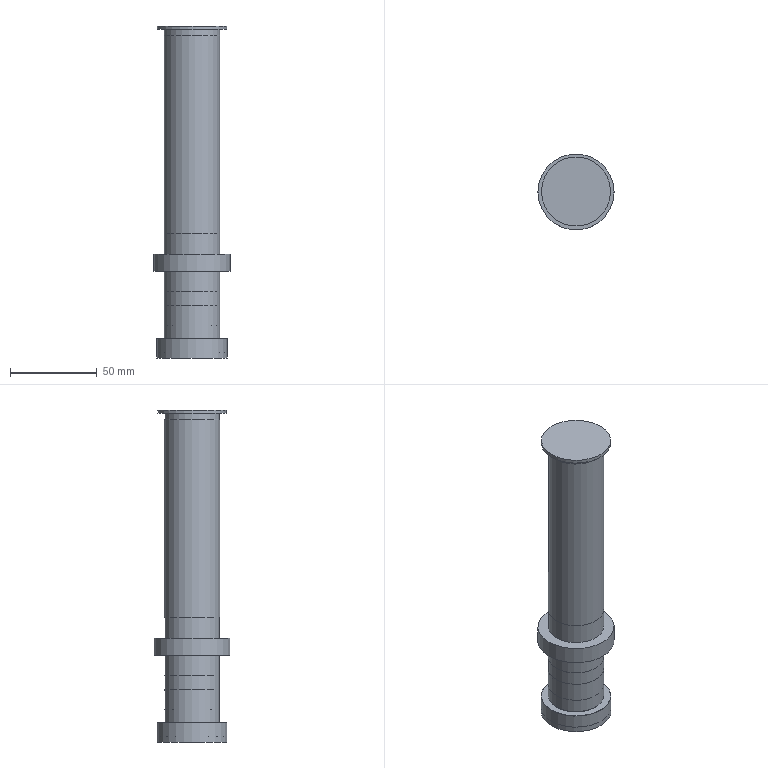Part | NX | features BREP 4 | 4 solids | 41 faces | box 44 x 44 x 191.85 mm | volume 315656 mm3 | plane 19 | cylinder 18 | torus 2 | cone 2 | commonest cylinder face diameters 8 x2 10 x2 14 x2 32 x2 40 x2 44 x2
STEP:
#1=CARTESIAN_POINT('',(-4.,0.,139.85));
#2=VERTEX_POINT('',#1);
#3=CARTESIAN_POINT('',(0.,0.,139.85));
#4=DIRECTION('',(0.,0.,1.));
#5=DIRECTION('',(-1.,0.,0.));
#6=AXIS2_PLACEMENT_3D('',#3,#4,#5);
#7=CIRCLE('',#6,4.);
#8=EDGE_CURVE('',#2,#2,#7,.T.);
#9=ORIENTED_EDGE('',*,*,#8,.F.);
#10=EDGE_LOOP('',(#9));
#11=FACE_BOUND('',#10,.T.);
#12=CARTESIAN_POINT('',(-4.,0.,134.85));
#13=VERTEX_POINT('',#12);
#14=CARTESIAN_POINT('',(0.,0.,134.85));
#15=DIRECTION('',(0.,0.,1.));
#16=DIRECTION('',(-1.,0.,0.));
#17=AXIS2_PLACEMENT_3D('',#14,#15,#16);
#18=CIRCLE('',#17,4.);
#19=EDGE_CURVE('',#13,#13,#18,.T.);
#20=ORIENTED_EDGE('',*,*,#19,.T.);
#21=EDGE_LOOP('',(#20));
#22=FACE_BOUND('',#21,.T.);
#23=CARTESIAN_POINT('',(0.,0.,139.85));
#24=DIRECTION('',(0.,0.,-1.));
#25=DIRECTION('',(1.,0.,0.));
#26=AXIS2_PLACEMENT_3D('',#23,#24,#25);
#27=CYLINDRICAL_SURFACE('',#26,4.);
#28=ADVANCED_FACE('',(#11,#22),#27,.T.);
#29=ORIENTED_EDGE('',*,*,#19,.F.);
#30=EDGE_LOOP('',(#29));
#31=FACE_BOUND('',#30,.T.);
#32=CARTESIAN_POINT('',(0.,0.,134.85));
#33=DIRECTION('',(0.,0.,1.));
#34=DIRECTION('',(-1.,0.,0.));
#35=AXIS2_PLACEMENT_3D('',#32,#33,#34);
#36=PLANE('',#35);
#37=ADVANCED_FACE('',(#31),#36,.F.);
#38=CARTESIAN_POINT('',(20.,0.,139.85));
#39=VERTEX_POINT('',#38);
#40=CARTESIAN_POINT('',(0.,0.,139.85));
#41=DIRECTION('',(0.,0.,1.));
#42=DIRECTION('',(1.,0.,0.));
#43=AXIS2_PLACEMENT_3D('',#40,#41,#42);
#44=CIRCLE('',#43,20.);
#45=EDGE_CURVE('',#39,#39,#44,.T.);
#46=ORIENTED_EDGE('',*,*,#45,.F.);
#47=EDGE_LOOP('',(#46));
#48=FACE_BOUND('',#47,.T.);
#49=ORIENTED_EDGE('',*,*,#8,.T.);
#50=EDGE_LOOP('',(#49));
#51=FACE_BOUND('',#50,.T.);
#52=CARTESIAN_POINT('',(0.,0.,139.85));
#53=DIRECTION('',(0.,0.,-1.));
#54=DIRECTION('',(1.,0.,0.));
#55=AXIS2_PLACEMENT_3D('',#52,#53,#54);
#56=PLANE('',#55);
#57=ADVANCED_FACE('',(#48,#51),#56,.T.);
#58=CARTESIAN_POINT('',(20.,0.,141.85));
#59=VERTEX_POINT('',#58);
#60=CARTESIAN_POINT('',(0.,0.,141.85));
#61=DIRECTION('',(0.,0.,1.));
#62=DIRECTION('',(1.,0.,0.));
#63=AXIS2_PLACEMENT_3D('',#60,#61,#62);
#64=CIRCLE('',#63,20.);
#65=EDGE_CURVE('',#59,#59,#64,.T.);
#66=ORIENTED_EDGE('',*,*,#65,.T.);
#67=EDGE_LOOP('',(#66));
#68=FACE_BOUND('',#67,.T.);
#69=CARTESIAN_POINT('',(0.,0.,141.85));
#70=DIRECTION('',(0.,0.,1.));
#71=DIRECTION('',(-1.,0.,0.));
#72=AXIS2_PLACEMENT_3D('',#69,#70,#71);
#73=PLANE('',#72);
#74=ADVANCED_FACE('',(#68),#73,.T.);
#75=ORIENTED_EDGE('',*,*,#65,.F.);
#76=EDGE_LOOP('',(#75));
#77=FACE_BOUND('',#76,.T.);
#78=ORIENTED_EDGE('',*,*,#45,.T.);
#79=EDGE_LOOP('',(#78));
#80=FACE_BOUND('',#79,.T.);
#81=CARTESIAN_POINT('',(0.,0.,139.85));
#82=DIRECTION('',(0.,0.,1.));
#83=DIRECTION('',(-1.,0.,0.));
#84=AXIS2_PLACEMENT_3D('',#81,#82,#83);
#85=CYLINDRICAL_SURFACE('',#84,20.);
#86=ADVANCED_FACE('',(#77,#80),#85,.T.);
#87=CLOSED_SHELL('',(#28,#37,#57,#74,#86));
#88=MANIFOLD_SOLID_BREP('',#87);
#89=CARTESIAN_POINT('',(16.,0.,0.));
#90=VERTEX_POINT('',#89);
#91=CARTESIAN_POINT('',(0.,0.,0.));
#92=DIRECTION('',(0.,0.,1.));
#93=DIRECTION('',(1.,0.,0.));
#94=AXIS2_PLACEMENT_3D('',#91,#92,#93);
#95=CIRCLE('',#94,16.);
#96=EDGE_CURVE('',#90,#90,#95,.T.);
#97=ORIENTED_EDGE('',*,*,#96,.F.);
#98=EDGE_LOOP('',(#97));
#99=FACE_BOUND('',#98,.T.);
#100=CARTESIAN_POINT('',(-16.,0.,-39.));
#101=VERTEX_POINT('',#100);
#102=CARTESIAN_POINT('',(0.,0.,-39.));
#103=DIRECTION('',(0.,0.,-1.));
#104=DIRECTION('',(-1.,0.,0.));
#105=AXIS2_PLACEMENT_3D('',#102,#103,#104);
#106=CIRCLE('',#105,16.);
#107=EDGE_CURVE('',#101,#101,#106,.T.);
#108=ORIENTED_EDGE('',*,*,#107,.F.);
#109=EDGE_LOOP('',(#108));
#110=FACE_BOUND('',#109,.T.);
#111=CARTESIAN_POINT('',(0.,0.,-23.));
#112=DIRECTION('',(0.,0.,1.));
#113=DIRECTION('',(-1.,0.,0.));
#114=AXIS2_PLACEMENT_3D('',#111,#112,#113);
#115=CYLINDRICAL_SURFACE('',#114,16.);
#116=ADVANCED_FACE('',(#99,#110),#115,.T.);
#117=CARTESIAN_POINT('',(-20.25,0.,-50.));
#118=VERTEX_POINT('',#117);
#119=CARTESIAN_POINT('',(0.,0.,-50.));
#120=DIRECTION('',(0.,0.,-1.));
#121=DIRECTION('',(-1.,0.,0.));
#122=AXIS2_PLACEMENT_3D('',#119,#120,#121);
#123=CIRCLE('',#122,20.25);
#124=EDGE_CURVE('',#118,#118,#123,.T.);
#125=ORIENTED_EDGE('',*,*,#124,.T.);
#126=EDGE_LOOP('',(#125));
#127=FACE_BOUND('',#126,.T.);
#128=CARTESIAN_POINT('',(0.,0.,-50.));
#129=DIRECTION('',(0.,0.,-1.));
#130=DIRECTION('',(1.,0.,0.));
#131=AXIS2_PLACEMENT_3D('',#128,#129,#130);
#132=PLANE('',#131);
#133=ADVANCED_FACE('',(#127),#132,.T.);
#134=ORIENTED_EDGE('',*,*,#107,.T.);
#135=EDGE_LOOP('',(#134));
#136=FACE_BOUND('',#135,.T.);
#137=CARTESIAN_POINT('',(-20.25,0.,-39.));
#138=VERTEX_POINT('',#137);
#139=CARTESIAN_POINT('',(0.,0.,-39.));
#140=DIRECTION('',(0.,0.,-1.));
#141=DIRECTION('',(-1.,0.,0.));
#142=AXIS2_PLACEMENT_3D('',#139,#140,#141);
#143=CIRCLE('',#142,20.25);
#144=EDGE_CURVE('',#138,#138,#143,.T.);
#145=ORIENTED_EDGE('',*,*,#144,.F.);
#146=EDGE_LOOP('',(#145));
#147=FACE_BOUND('',#146,.T.);
#148=CARTESIAN_POINT('',(0.,0.,-39.));
#149=DIRECTION('',(0.,0.,1.));
#150=DIRECTION('',(-1.,0.,0.));
#151=AXIS2_PLACEMENT_3D('',#148,#149,#150);
#152=PLANE('',#151);
#153=ADVANCED_FACE('',(#136,#147),#152,.T.);
#154=ORIENTED_EDGE('',*,*,#124,.F.);
#155=EDGE_LOOP('',(#154));
#156=FACE_BOUND('',#155,.T.);
#157=ORIENTED_EDGE('',*,*,#144,.T.);
#158=EDGE_LOOP('',(#157));
#159=FACE_BOUND('',#158,.T.);
#160=CARTESIAN_POINT('',(0.,0.,-39.));
#161=DIRECTION('',(0.,0.,-1.));
#162=DIRECTION('',(1.,0.,0.));
#163=AXIS2_PLACEMENT_3D('',#160,#161,#162);
#164=CYLINDRICAL_SURFACE('',#163,20.25);
#165=ADVANCED_FACE('',(#156,#159),#164,.T.);
#166=CARTESIAN_POINT('',(16.,0.,10.));
#167=VERTEX_POINT('',#166);
#168=CARTESIAN_POINT('',(0.,0.,10.));
#169=DIRECTION('',(0.,0.,1.));
#170=DIRECTION('',(1.,0.,0.));
#171=AXIS2_PLACEMENT_3D('',#168,#169,#170);
#172=CIRCLE('',#171,16.);
#173=EDGE_CURVE('',#167,#167,#172,.T.);
#174=ORIENTED_EDGE('',*,*,#173,.F.);
#175=EDGE_LOOP('',(#174));
#176=FACE_BOUND('',#175,.T.);
#177=CARTESIAN_POINT('',(22.,0.,10.));
#178=VERTEX_POINT('',#177);
#179=CARTESIAN_POINT('',(0.,0.,10.));
#180=DIRECTION('',(0.,0.,1.));
#181=DIRECTION('',(1.,0.,0.));
#182=AXIS2_PLACEMENT_3D('',#179,#180,#181);
#183=CIRCLE('',#182,22.);
#184=EDGE_CURVE('',#178,#178,#183,.T.);
#185=ORIENTED_EDGE('',*,*,#184,.T.);
#186=EDGE_LOOP('',(#185));
#187=FACE_BOUND('',#186,.T.);
#188=CARTESIAN_POINT('',(0.,0.,10.));
#189=DIRECTION('',(0.,0.,1.));
#190=DIRECTION('',(-1.,0.,0.));
#191=AXIS2_PLACEMENT_3D('',#188,#189,#190);
#192=PLANE('',#191);
#193=ADVANCED_FACE('',(#176,#187),#192,.T.);
#194=ORIENTED_EDGE('',*,*,#96,.T.);
#195=EDGE_LOOP('',(#194));
#196=FACE_BOUND('',#195,.T.);
#197=CARTESIAN_POINT('',(22.,0.,0.));
#198=VERTEX_POINT('',#197);
#199=CARTESIAN_POINT('',(0.,0.,0.));
#200=DIRECTION('',(0.,0.,1.));
#201=DIRECTION('',(1.,0.,0.));
#202=AXIS2_PLACEMENT_3D('',#199,#200,#201);
#203=CIRCLE('',#202,22.);
#204=EDGE_CURVE('',#198,#198,#203,.T.);
#205=ORIENTED_EDGE('',*,*,#204,.F.);
#206=EDGE_LOOP('',(#205));
#207=FACE_BOUND('',#206,.T.);
#208=CARTESIAN_POINT('',(0.,0.,0.));
#209=DIRECTION('',(0.,0.,-1.));
#210=DIRECTION('',(1.,0.,0.));
#211=AXIS2_PLACEMENT_3D('',#208,#209,#210);
#212=PLANE('',#211);
#213=ADVANCED_FACE('',(#196,#207),#212,.T.);
#214=ORIENTED_EDGE('',*,*,#184,.F.);
#215=EDGE_LOOP('',(#214));
#216=FACE_BOUND('',#215,.T.);
#217=ORIENTED_EDGE('',*,*,#204,.T.);
#218=EDGE_LOOP('',(#217));
#219=FACE_BOUND('',#218,.T.);
#220=CARTESIAN_POINT('',(0.,0.,0.));
#221=DIRECTION('',(0.,0.,1.));
#222=DIRECTION('',(-1.,0.,0.));
#223=AXIS2_PLACEMENT_3D('',#220,#221,#222);
#224=CYLINDRICAL_SURFACE('',#223,22.);
#225=ADVANCED_FACE('',(#216,#219),#224,.T.);
#226=CARTESIAN_POINT('',(16.,0.,139.85));
#227=VERTEX_POINT('',#226);
#228=CARTESIAN_POINT('',(0.,0.,139.85));
#229=DIRECTION('',(0.,0.,1.));
#230=DIRECTION('',(1.,0.,0.));
#231=AXIS2_PLACEMENT_3D('',#228,#229,#230);
#232=CIRCLE('',#231,16.);
#233=EDGE_CURVE('',#227,#227,#232,.T.);
#234=ORIENTED_EDGE('',*,*,#233,.T.);
#235=EDGE_LOOP('',(#234));
#236=FACE_BOUND('',#235,.T.);
#237=CARTESIAN_POINT('',(0.,0.,139.85));
#238=DIRECTION('',(0.,0.,1.));
#239=DIRECTION('',(-1.,0.,0.));
#240=AXIS2_PLACEMENT_3D('',#237,#238,#239);
#241=PLANE('',#240);
#242=ADVANCED_FACE('',(#236),#241,.T.);
#243=ORIENTED_EDGE('',*,*,#233,.F.);
#244=EDGE_LOOP('',(#243));
#245=FACE_BOUND('',#244,.T.);
#246=ORIENTED_EDGE('',*,*,#173,.T.);
#247=EDGE_LOOP('',(#246));
#248=FACE_BOUND('',#247,.T.);
#249=CARTESIAN_POINT('',(0.,0.,10.));
#250=DIRECTION('',(0.,0.,1.));
#251=DIRECTION('',(-1.,0.,0.));
#252=AXIS2_PLACEMENT_3D('',#249,#250,#251);
#253=CYLINDRICAL_SURFACE('',#252,16.);
#254=ADVANCED_FACE('',(#245,#248),#253,.T.);
#255=CLOSED_SHELL('',(#116,#133,#153,#165,#193,#213,#225,#242,#254));
#256=MANIFOLD_SOLID_BREP('',#255);
#257=CARTESIAN_POINT('',(-7.,0.,139.85));
#258=VERTEX_POINT('',#257);
#259=CARTESIAN_POINT('',(0.,0.,139.85));
#260=DIRECTION('',(0.,0.,-1.));
#261=DIRECTION('',(-1.,0.,0.));
#262=AXIS2_PLACEMENT_3D('',#259,#260,#261);
#263=CIRCLE('',#262,7.);
#264=EDGE_CURVE('',#258,#258,#263,.T.);
#265=ORIENTED_EDGE('',*,*,#264,.T.);
#266=EDGE_LOOP('',(#265));
#267=FACE_BOUND('',#266,.T.);
#268=CARTESIAN_POINT('',(12.509,0.,139.85));
#269=VERTEX_POINT('',#268);
#270=CARTESIAN_POINT('',(0.,0.,139.85));
#271=DIRECTION('',(0.,0.,1.));
#272=DIRECTION('',(1.,0.,0.));
#273=AXIS2_PLACEMENT_3D('',#270,#271,#272);
#274=CIRCLE('',#273,12.509);
#275=EDGE_CURVE('',#269,#269,#274,.T.);
#276=ORIENTED_EDGE('',*,*,#275,.T.);
#277=EDGE_LOOP('',(#276));
#278=FACE_BOUND('',#277,.T.);
#279=CARTESIAN_POINT('',(0.,0.,139.85));
#280=DIRECTION('',(0.,0.,1.));
#281=DIRECTION('',(-1.,0.,0.));
#282=AXIS2_PLACEMENT_3D('',#279,#280,#281);
#283=PLANE('',#282);
#284=ADVANCED_FACE('',(#267,#278),#283,.T.);
#285=CARTESIAN_POINT('',(16.009,0.,22.));
#286=VERTEX_POINT('',#285);
#287=CARTESIAN_POINT('',(0.,0.,22.));
#288=DIRECTION('',(0.,0.,-1.));
#289=DIRECTION('',(1.,0.,0.));
#290=AXIS2_PLACEMENT_3D('',#287,#288,#289);
#291=CIRCLE('',#290,16.009);
#292=EDGE_CURVE('',#286,#286,#291,.T.);
#293=ORIENTED_EDGE('',*,*,#292,.F.);
#294=EDGE_LOOP('',(#293));
#295=FACE_BOUND('',#294,.T.);
#296=CARTESIAN_POINT('',(16.009,0.,136.35));
#297=VERTEX_POINT('',#296);
#298=CARTESIAN_POINT('',(0.,0.,136.35));
#299=DIRECTION('',(0.,0.,-1.));
#300=DIRECTION('',(1.,0.,0.));
#301=AXIS2_PLACEMENT_3D('',#298,#299,#300);
#302=CIRCLE('',#301,16.009);
#303=EDGE_CURVE('',#297,#297,#302,.T.);
#304=ORIENTED_EDGE('',*,*,#303,.T.);
#305=EDGE_LOOP('',(#304));
#306=FACE_BOUND('',#305,.T.);
#307=CARTESIAN_POINT('',(0.,0.,10.));
#308=DIRECTION('',(0.,0.,1.));
#309=DIRECTION('',(-1.,0.,0.));
#310=AXIS2_PLACEMENT_3D('',#307,#308,#309);
#311=CYLINDRICAL_SURFACE('',#310,16.009);
#312=ADVANCED_FACE('',(#295,#306),#311,.T.);
#313=ORIENTED_EDGE('',*,*,#303,.F.);
#314=EDGE_LOOP('',(#313));
#315=FACE_BOUND('',#314,.T.);
#316=ORIENTED_EDGE('',*,*,#275,.F.);
#317=EDGE_LOOP('',(#316));
#318=FACE_BOUND('',#317,.T.);
#319=CARTESIAN_POINT('',(0.,0.,136.35));
#320=DIRECTION('',(0.,0.,1.));
#321=DIRECTION('',(-1.,0.,0.));
#322=AXIS2_PLACEMENT_3D('',#319,#320,#321);
#323=TOROIDAL_SURFACE('',#322,12.509,3.5);
#324=ADVANCED_FACE('',(#315,#318),#323,.T.);
#325=CARTESIAN_POINT('',(-4.,0.,114.85));
#326=VERTEX_POINT('',#325);
#327=CARTESIAN_POINT('',(0.,0.,114.85));
#328=DIRECTION('',(0.,0.,-1.));
#329=DIRECTION('',(-1.,0.,0.));
#330=AXIS2_PLACEMENT_3D('',#327,#328,#329);
#331=CIRCLE('',#330,4.);
#332=EDGE_CURVE('',#326,#326,#331,.T.);
#333=ORIENTED_EDGE('',*,*,#332,.F.);
#334=EDGE_LOOP('',(#333));
#335=FACE_BOUND('',#334,.T.);
#336=CARTESIAN_POINT('',(0.,0.,112.447));
#337=VERTEX_POINT('',#336);
#338=VERTEX_LOOP('',#337);
#339=FACE_BOUND('',#338,.T.);
#340=CARTESIAN_POINT('',(0.,0.,114.85));
#341=DIRECTION('',(0.,0.,1.));
#342=DIRECTION('',(-1.,0.,0.));
#343=AXIS2_PLACEMENT_3D('',#340,#341,#342);
#344=CONICAL_SURFACE('',#343,4.,1.03);
#345=ADVANCED_FACE('',(#335,#339),#344,.F.);
#346=ORIENTED_EDGE('',*,*,#332,.T.);
#347=EDGE_LOOP('',(#346));
#348=FACE_BOUND('',#347,.T.);
#349=CARTESIAN_POINT('',(-4.,0.,134.85));
#350=VERTEX_POINT('',#349);
#351=CARTESIAN_POINT('',(0.,0.,134.85));
#352=DIRECTION('',(0.,0.,-1.));
#353=DIRECTION('',(-1.,0.,0.));
#354=AXIS2_PLACEMENT_3D('',#351,#352,#353);
#355=CIRCLE('',#354,4.);
#356=EDGE_CURVE('',#350,#350,#355,.T.);
#357=ORIENTED_EDGE('',*,*,#356,.F.);
#358=EDGE_LOOP('',(#357));
#359=FACE_BOUND('',#358,.T.);
#360=CARTESIAN_POINT('',(0.,0.,114.85));
#361=DIRECTION('',(0.,0.,-1.));
#362=DIRECTION('',(1.,0.,0.));
#363=AXIS2_PLACEMENT_3D('',#360,#361,#362);
#364=CYLINDRICAL_SURFACE('',#363,4.);
#365=ADVANCED_FACE('',(#348,#359),#364,.F.);
#366=ORIENTED_EDGE('',*,*,#356,.T.);
#367=EDGE_LOOP('',(#366));
#368=FACE_BOUND('',#367,.T.);
#369=CARTESIAN_POINT('',(-7.,0.,134.85));
#370=VERTEX_POINT('',#369);
#371=CARTESIAN_POINT('',(0.,0.,134.85));
#372=DIRECTION('',(0.,0.,-1.));
#373=DIRECTION('',(-1.,0.,0.));
#374=AXIS2_PLACEMENT_3D('',#371,#372,#373);
#375=CIRCLE('',#374,7.);
#376=EDGE_CURVE('',#370,#370,#375,.T.);
#377=ORIENTED_EDGE('',*,*,#376,.F.);
#378=EDGE_LOOP('',(#377));
#379=FACE_BOUND('',#378,.T.);
#380=CARTESIAN_POINT('',(0.,0.,134.85));
#381=DIRECTION('',(0.,0.,-1.));
#382=DIRECTION('',(1.,0.,0.));
#383=AXIS2_PLACEMENT_3D('',#380,#381,#382);
#384=PLANE('',#383);
#385=ADVANCED_FACE('',(#368,#379),#384,.F.);
#386=ORIENTED_EDGE('',*,*,#376,.T.);
#387=EDGE_LOOP('',(#386));
#388=FACE_BOUND('',#387,.T.);
#389=ORIENTED_EDGE('',*,*,#264,.F.);
#390=EDGE_LOOP('',(#389));
#391=FACE_BOUND('',#390,.T.);
#392=CARTESIAN_POINT('',(0.,0.,139.85));
#393=DIRECTION('',(0.,0.,-1.));
#394=DIRECTION('',(1.,0.,0.));
#395=AXIS2_PLACEMENT_3D('',#392,#393,#394);
#396=CYLINDRICAL_SURFACE('',#395,7.);
#397=ADVANCED_FACE('',(#388,#391),#396,.F.);
#398=CARTESIAN_POINT('',(15.208,0.,22.));
#399=VERTEX_POINT('',#398);
#400=CARTESIAN_POINT('',(0.,0.,22.));
#401=DIRECTION('',(0.,0.,1.));
#402=DIRECTION('',(1.,0.,0.));
#403=AXIS2_PLACEMENT_3D('',#400,#401,#402);
#404=CIRCLE('',#403,15.208);
#405=EDGE_CURVE('',#399,#399,#404,.T.);
#406=ORIENTED_EDGE('',*,*,#405,.F.);
#407=EDGE_LOOP('',(#406));
#408=FACE_BOUND('',#407,.T.);
#409=CARTESIAN_POINT('',(15.208,0.,10.));
#410=VERTEX_POINT('',#409);
#411=CARTESIAN_POINT('',(0.,0.,10.));
#412=DIRECTION('',(0.,0.,1.));
#413=DIRECTION('',(1.,0.,0.));
#414=AXIS2_PLACEMENT_3D('',#411,#412,#413);
#415=CIRCLE('',#414,15.208);
#416=EDGE_CURVE('',#410,#410,#415,.T.);
#417=ORIENTED_EDGE('',*,*,#416,.T.);
#418=EDGE_LOOP('',(#417));
#419=FACE_BOUND('',#418,.T.);
#420=CARTESIAN_POINT('',(0.,0.,16.));
#421=DIRECTION('',(0.,0.,1.));
#422=DIRECTION('',(-1.,0.,0.));
#423=AXIS2_PLACEMENT_3D('',#420,#421,#422);
#424=CYLINDRICAL_SURFACE('',#423,15.208);
#425=ADVANCED_FACE('',(#408,#419),#424,.T.);
#426=ORIENTED_EDGE('',*,*,#292,.T.);
#427=EDGE_LOOP('',(#426));
#428=FACE_BOUND('',#427,.T.);
#429=ORIENTED_EDGE('',*,*,#405,.T.);
#430=EDGE_LOOP('',(#429));
#431=FACE_BOUND('',#430,.T.);
#432=CARTESIAN_POINT('',(0.,0.,22.));
#433=DIRECTION('',(0.,0.,1.));
#434=DIRECTION('',(-1.,0.,0.));
#435=AXIS2_PLACEMENT_3D('',#432,#433,#434);
#436=PLANE('',#435);
#437=ADVANCED_FACE('',(#428,#431),#436,.F.);
#438=CARTESIAN_POINT('',(-15.999,0.,0.));
#439=VERTEX_POINT('',#438);
#440=CARTESIAN_POINT('',(0.,0.,0.));
#441=DIRECTION('',(0.,0.,-1.));
#442=DIRECTION('',(-1.,0.,0.));
#443=AXIS2_PLACEMENT_3D('',#440,#441,#442);
#444=CIRCLE('',#443,15.999);
#445=EDGE_CURVE('',#439,#439,#444,.T.);
#446=ORIENTED_EDGE('',*,*,#445,.F.);
#447=EDGE_LOOP('',(#446));
#448=FACE_BOUND('',#447,.T.);
#449=CARTESIAN_POINT('',(22.,0.,0.));
#450=VERTEX_POINT('',#449);
#451=CARTESIAN_POINT('',(0.,0.,0.));
#452=DIRECTION('',(0.,0.,1.));
#453=DIRECTION('',(1.,0.,0.));
#454=AXIS2_PLACEMENT_3D('',#451,#452,#453);
#455=CIRCLE('',#454,22.);
#456=EDGE_CURVE('',#450,#450,#455,.T.);
#457=ORIENTED_EDGE('',*,*,#456,.F.);
#458=EDGE_LOOP('',(#457));
#459=FACE_BOUND('',#458,.T.);
#460=CARTESIAN_POINT('',(0.,0.,0.));
#461=DIRECTION('',(0.,0.,1.));
#462=DIRECTION('',(-1.,0.,0.));
#463=AXIS2_PLACEMENT_3D('',#460,#461,#462);
#464=PLANE('',#463);
#465=ADVANCED_FACE('',(#448,#459),#464,.F.);
#466=CARTESIAN_POINT('',(22.,0.,10.));
#467=VERTEX_POINT('',#466);
#468=CARTESIAN_POINT('',(0.,0.,10.));
#469=DIRECTION('',(0.,0.,1.));
#470=DIRECTION('',(1.,0.,0.));
#471=AXIS2_PLACEMENT_3D('',#468,#469,#470);
#472=CIRCLE('',#471,22.);
#473=EDGE_CURVE('',#467,#467,#472,.T.);
#474=ORIENTED_EDGE('',*,*,#473,.F.);
#475=EDGE_LOOP('',(#474));
#476=FACE_BOUND('',#475,.T.);
#477=ORIENTED_EDGE('',*,*,#456,.T.);
#478=EDGE_LOOP('',(#477));
#479=FACE_BOUND('',#478,.T.);
#480=CARTESIAN_POINT('',(0.,0.,10.));
#481=DIRECTION('',(0.,0.,-1.));
#482=DIRECTION('',(1.,0.,0.));
#483=AXIS2_PLACEMENT_3D('',#480,#481,#482);
#484=CYLINDRICAL_SURFACE('',#483,22.);
#485=ADVANCED_FACE('',(#476,#479),#484,.T.);
#486=ORIENTED_EDGE('',*,*,#473,.T.);
#487=EDGE_LOOP('',(#486));
#488=FACE_BOUND('',#487,.T.);
#489=ORIENTED_EDGE('',*,*,#416,.F.);
#490=EDGE_LOOP('',(#489));
#491=FACE_BOUND('',#490,.T.);
#492=CARTESIAN_POINT('',(0.,0.,10.));
#493=DIRECTION('',(0.,0.,1.));
#494=DIRECTION('',(-1.,0.,0.));
#495=AXIS2_PLACEMENT_3D('',#492,#493,#494);
#496=PLANE('',#495);
#497=ADVANCED_FACE('',(#488,#491),#496,.T.);
#498=CARTESIAN_POINT('',(-15.98,0.,-11.5));
#499=VERTEX_POINT('',#498);
#500=CARTESIAN_POINT('',(0.,0.,-11.5));
#501=DIRECTION('',(0.,0.,-1.));
#502=DIRECTION('',(-1.,0.,0.));
#503=AXIS2_PLACEMENT_3D('',#500,#501,#502);
#504=CIRCLE('',#503,15.98);
#505=EDGE_CURVE('',#499,#499,#504,.T.);
#506=ORIENTED_EDGE('',*,*,#505,.F.);
#507=EDGE_LOOP('',(#506));
#508=FACE_BOUND('',#507,.T.);
#509=CARTESIAN_POINT('',(-15.999,0.,-11.5));
#510=VERTEX_POINT('',#509);
#511=CARTESIAN_POINT('',(0.,0.,-11.5));
#512=DIRECTION('',(0.,0.,-1.));
#513=DIRECTION('',(-1.,0.,0.));
#514=AXIS2_PLACEMENT_3D('',#511,#512,#513);
#515=CIRCLE('',#514,15.999);
#516=EDGE_CURVE('',#510,#510,#515,.T.);
#517=ORIENTED_EDGE('',*,*,#516,.T.);
#518=EDGE_LOOP('',(#517));
#519=FACE_BOUND('',#518,.T.);
#520=CARTESIAN_POINT('',(0.,0.,-11.5));
#521=DIRECTION('',(0.,0.,-1.));
#522=DIRECTION('',(1.,0.,0.));
#523=AXIS2_PLACEMENT_3D('',#520,#521,#522);
#524=PLANE('',#523);
#525=ADVANCED_FACE('',(#508,#519),#524,.T.);
#526=ORIENTED_EDGE('',*,*,#516,.F.);
#527=EDGE_LOOP('',(#526));
#528=FACE_BOUND('',#527,.T.);
#529=ORIENTED_EDGE('',*,*,#445,.T.);
#530=EDGE_LOOP('',(#529));
#531=FACE_BOUND('',#530,.T.);
#532=CARTESIAN_POINT('',(0.,0.,0.));
#533=DIRECTION('',(0.,0.,-1.));
#534=DIRECTION('',(1.,0.,0.));
#535=AXIS2_PLACEMENT_3D('',#532,#533,#534);
#536=CYLINDRICAL_SURFACE('',#535,15.999);
#537=ADVANCED_FACE('',(#528,#531),#536,.T.);
#538=CARTESIAN_POINT('',(5.,0.,-23.));
#539=VERTEX_POINT('',#538);
#540=CARTESIAN_POINT('',(0.,0.,-23.));
#541=DIRECTION('',(0.,0.,1.));
#542=DIRECTION('',(1.,0.,0.));
#543=AXIS2_PLACEMENT_3D('',#540,#541,#542);
#544=CIRCLE('',#543,5.);
#545=EDGE_CURVE('',#539,#539,#544,.T.);
#546=ORIENTED_EDGE('',*,*,#545,.T.);
#547=EDGE_LOOP('',(#546));
#548=FACE_BOUND('',#547,.T.);
#549=CARTESIAN_POINT('',(-12.48,0.,-23.));
#550=VERTEX_POINT('',#549);
#551=CARTESIAN_POINT('',(0.,0.,-23.));
#552=DIRECTION('',(0.,0.,-1.));
#553=DIRECTION('',(-1.,0.,0.));
#554=AXIS2_PLACEMENT_3D('',#551,#552,#553);
#555=CIRCLE('',#554,12.48);
#556=EDGE_CURVE('',#550,#550,#555,.T.);
#557=ORIENTED_EDGE('',*,*,#556,.T.);
#558=EDGE_LOOP('',(#557));
#559=FACE_BOUND('',#558,.T.);
#560=CARTESIAN_POINT('',(0.,0.,-23.));
#561=DIRECTION('',(0.,0.,-1.));
#562=DIRECTION('',(1.,0.,0.));
#563=AXIS2_PLACEMENT_3D('',#560,#561,#562);
#564=PLANE('',#563);
#565=ADVANCED_FACE('',(#548,#559),#564,.T.);
#566=CARTESIAN_POINT('',(-15.98,0.,-19.5));
#567=VERTEX_POINT('',#566);
#568=CARTESIAN_POINT('',(0.,0.,-19.5));
#569=DIRECTION('',(0.,0.,1.));
#570=DIRECTION('',(-1.,0.,0.));
#571=AXIS2_PLACEMENT_3D('',#568,#569,#570);
#572=CIRCLE('',#571,15.98);
#573=EDGE_CURVE('',#567,#567,#572,.T.);
#574=ORIENTED_EDGE('',*,*,#573,.T.);
#575=EDGE_LOOP('',(#574));
#576=FACE_BOUND('',#575,.T.);
#577=ORIENTED_EDGE('',*,*,#505,.T.);
#578=EDGE_LOOP('',(#577));
#579=FACE_BOUND('',#578,.T.);
#580=CARTESIAN_POINT('',(0.,0.,-11.5));
#581=DIRECTION('',(0.,0.,-1.));
#582=DIRECTION('',(1.,0.,0.));
#583=AXIS2_PLACEMENT_3D('',#580,#581,#582);
#584=CYLINDRICAL_SURFACE('',#583,15.98);
#585=ADVANCED_FACE('',(#576,#579),#584,.T.);
#586=ORIENTED_EDGE('',*,*,#573,.F.);
#587=EDGE_LOOP('',(#586));
#588=FACE_BOUND('',#587,.T.);
#589=ORIENTED_EDGE('',*,*,#556,.F.);
#590=EDGE_LOOP('',(#589));
#591=FACE_BOUND('',#590,.T.);
#592=CARTESIAN_POINT('',(0.,0.,-19.5));
#593=DIRECTION('',(0.,0.,-1.));
#594=DIRECTION('',(1.,0.,0.));
#595=AXIS2_PLACEMENT_3D('',#592,#593,#594);
#596=TOROIDAL_SURFACE('',#595,12.48,3.5);
#597=ADVANCED_FACE('',(#588,#591),#596,.T.);
#598=CARTESIAN_POINT('',(5.,0.,-4.6));
#599=VERTEX_POINT('',#598);
#600=CARTESIAN_POINT('',(0.,0.,-4.6));
#601=DIRECTION('',(0.,0.,1.));
#602=DIRECTION('',(1.,0.,0.));
#603=AXIS2_PLACEMENT_3D('',#600,#601,#602);
#604=CIRCLE('',#603,5.);
#605=EDGE_CURVE('',#599,#599,#604,.T.);
#606=ORIENTED_EDGE('',*,*,#605,.F.);
#607=EDGE_LOOP('',(#606));
#608=FACE_BOUND('',#607,.T.);
#609=CARTESIAN_POINT('',(0.,0.,-1.596));
#610=VERTEX_POINT('',#609);
#611=VERTEX_LOOP('',#610);
#612=FACE_BOUND('',#611,.T.);
#613=CARTESIAN_POINT('',(0.,0.,-4.6));
#614=DIRECTION('',(0.,0.,-1.));
#615=DIRECTION('',(1.,0.,0.));
#616=AXIS2_PLACEMENT_3D('',#613,#614,#615);
#617=CONICAL_SURFACE('',#616,5.,1.03);
#618=ADVANCED_FACE('',(#608,#612),#617,.F.);
#619=ORIENTED_EDGE('',*,*,#605,.T.);
#620=EDGE_LOOP('',(#619));
#621=FACE_BOUND('',#620,.T.);
#622=ORIENTED_EDGE('',*,*,#545,.F.);
#623=EDGE_LOOP('',(#622));
#624=FACE_BOUND('',#623,.T.);
#625=CARTESIAN_POINT('',(0.,0.,-23.));
#626=DIRECTION('',(0.,0.,1.));
#627=DIRECTION('',(-1.,0.,0.));
#628=AXIS2_PLACEMENT_3D('',#625,#626,#627);
#629=CYLINDRICAL_SURFACE('',#628,5.);
#630=ADVANCED_FACE('',(#621,#624),#629,.F.);
#631=CLOSED_SHELL('',(#284,#312,#324,#345,#365,#385,#397,#425,#437,#465,#485,#497,#525,#537,#565,#585,#597,#618,#630));
#632=MANIFOLD_SOLID_BREP('',#631);
#633=CARTESIAN_POINT('',(20.,0.,-39.));
#634=VERTEX_POINT('',#633);
#635=CARTESIAN_POINT('',(0.,0.,-39.));
#636=DIRECTION('',(0.,0.,1.));
#637=DIRECTION('',(1.,0.,0.));
#638=AXIS2_PLACEMENT_3D('',#635,#636,#637);
#639=CIRCLE('',#638,20.);
#640=EDGE_CURVE('',#634,#634,#639,.T.);
#641=ORIENTED_EDGE('',*,*,#640,.F.);
#642=EDGE_LOOP('',(#641));
#643=FACE_BOUND('',#642,.T.);
#644=CARTESIAN_POINT('',(20.,0.,-47.));
#645=VERTEX_POINT('',#644);
#646=CARTESIAN_POINT('',(0.,0.,-47.));
#647=DIRECTION('',(0.,0.,1.));
#648=DIRECTION('',(1.,0.,0.));
#649=AXIS2_PLACEMENT_3D('',#646,#647,#648);
#650=CIRCLE('',#649,20.);
#651=EDGE_CURVE('',#645,#645,#650,.T.);
#652=ORIENTED_EDGE('',*,*,#651,.T.);
#653=EDGE_LOOP('',(#652));
#654=FACE_BOUND('',#653,.T.);
#655=CARTESIAN_POINT('',(0.,0.,-39.));
#656=DIRECTION('',(0.,0.,-1.));
#657=DIRECTION('',(1.,0.,0.));
#658=AXIS2_PLACEMENT_3D('',#655,#656,#657);
#659=CYLINDRICAL_SURFACE('',#658,20.);
#660=ADVANCED_FACE('',(#643,#654),#659,.T.);
#661=CARTESIAN_POINT('',(15.75,0.,-39.));
#662=VERTEX_POINT('',#661);
#663=CARTESIAN_POINT('',(0.,0.,-39.));
#664=DIRECTION('',(0.,0.,1.));
#665=DIRECTION('',(1.,0.,0.));
#666=AXIS2_PLACEMENT_3D('',#663,#664,#665);
#667=CIRCLE('',#666,15.75);
#668=EDGE_CURVE('',#662,#662,#667,.T.);
#669=ORIENTED_EDGE('',*,*,#668,.F.);
#670=EDGE_LOOP('',(#669));
#671=FACE_BOUND('',#670,.T.);
#672=ORIENTED_EDGE('',*,*,#640,.T.);
#673=EDGE_LOOP('',(#672));
#674=FACE_BOUND('',#673,.T.);
#675=CARTESIAN_POINT('',(0.,0.,-39.));
#676=DIRECTION('',(0.,0.,1.));
#677=DIRECTION('',(-1.,0.,0.));
#678=AXIS2_PLACEMENT_3D('',#675,#676,#677);
#679=PLANE('',#678);
#680=ADVANCED_FACE('',(#671,#674),#679,.T.);
#681=CARTESIAN_POINT('',(7.,0.,-47.));
#682=VERTEX_POINT('',#681);
#683=CARTESIAN_POINT('',(0.,0.,-47.));
#684=DIRECTION('',(0.,0.,1.));
#685=DIRECTION('',(1.,0.,0.));
#686=AXIS2_PLACEMENT_3D('',#683,#684,#685);
#687=CIRCLE('',#686,7.);
#688=EDGE_CURVE('',#682,#682,#687,.T.);
#689=ORIENTED_EDGE('',*,*,#688,.T.);
#690=EDGE_LOOP('',(#689));
#691=FACE_BOUND('',#690,.T.);
#692=ORIENTED_EDGE('',*,*,#651,.F.);
#693=EDGE_LOOP('',(#692));
#694=FACE_BOUND('',#693,.T.);
#695=CARTESIAN_POINT('',(0.,0.,-47.));
#696=DIRECTION('',(0.,0.,1.));
#697=DIRECTION('',(-1.,0.,0.));
#698=AXIS2_PLACEMENT_3D('',#695,#696,#697);
#699=PLANE('',#698);
#700=ADVANCED_FACE('',(#691,#694),#699,.F.);
#701=CARTESIAN_POINT('',(5.,0.,-31.));
#702=VERTEX_POINT('',#701);
#703=CARTESIAN_POINT('',(0.,0.,-31.));
#704=DIRECTION('',(0.,0.,1.));
#705=DIRECTION('',(1.,0.,0.));
#706=AXIS2_PLACEMENT_3D('',#703,#704,#705);
#707=CIRCLE('',#706,5.);
#708=EDGE_CURVE('',#702,#702,#707,.T.);
#709=ORIENTED_EDGE('',*,*,#708,.F.);
#710=EDGE_LOOP('',(#709));
#711=FACE_BOUND('',#710,.T.);
#712=CARTESIAN_POINT('',(15.75,0.,-31.));
#713=VERTEX_POINT('',#712);
#714=CARTESIAN_POINT('',(0.,0.,-31.));
#715=DIRECTION('',(0.,0.,1.));
#716=DIRECTION('',(1.,0.,0.));
#717=AXIS2_PLACEMENT_3D('',#714,#715,#716);
#718=CIRCLE('',#717,15.75);
#719=EDGE_CURVE('',#713,#713,#718,.T.);
#720=ORIENTED_EDGE('',*,*,#719,.T.);
#721=EDGE_LOOP('',(#720));
#722=FACE_BOUND('',#721,.T.);
#723=CARTESIAN_POINT('',(0.,0.,-31.));
#724=DIRECTION('',(0.,0.,1.));
#725=DIRECTION('',(-1.,0.,0.));
#726=AXIS2_PLACEMENT_3D('',#723,#724,#725);
#727=PLANE('',#726);
#728=ADVANCED_FACE('',(#711,#722),#727,.T.);
#729=ORIENTED_EDGE('',*,*,#719,.F.);
#730=EDGE_LOOP('',(#729));
#731=FACE_BOUND('',#730,.T.);
#732=ORIENTED_EDGE('',*,*,#668,.T.);
#733=EDGE_LOOP('',(#732));
#734=FACE_BOUND('',#733,.T.);
#735=CARTESIAN_POINT('',(0.,0.,-39.));
#736=DIRECTION('',(0.,0.,1.));
#737=DIRECTION('',(-1.,0.,0.));
#738=AXIS2_PLACEMENT_3D('',#735,#736,#737);
#739=CYLINDRICAL_SURFACE('',#738,15.75);
#740=ADVANCED_FACE('',(#731,#734),#739,.T.);
#741=ORIENTED_EDGE('',*,*,#708,.T.);
#742=EDGE_LOOP('',(#741));
#743=FACE_BOUND('',#742,.T.);
#744=CARTESIAN_POINT('',(5.,0.,-37.));
#745=VERTEX_POINT('',#744);
#746=CARTESIAN_POINT('',(0.,0.,-37.));
#747=DIRECTION('',(0.,0.,1.));
#748=DIRECTION('',(1.,0.,0.));
#749=AXIS2_PLACEMENT_3D('',#746,#747,#748);
#750=CIRCLE('',#749,5.);
#751=EDGE_CURVE('',#745,#745,#750,.T.);
#752=ORIENTED_EDGE('',*,*,#751,.F.);
#753=EDGE_LOOP('',(#752));
#754=FACE_BOUND('',#753,.T.);
#755=CARTESIAN_POINT('',(0.,0.,-31.));
#756=DIRECTION('',(0.,0.,1.));
#757=DIRECTION('',(-1.,0.,0.));
#758=AXIS2_PLACEMENT_3D('',#755,#756,#757);
#759=CYLINDRICAL_SURFACE('',#758,5.);
#760=ADVANCED_FACE('',(#743,#754),#759,.F.);
#761=ORIENTED_EDGE('',*,*,#751,.T.);
#762=EDGE_LOOP('',(#761));
#763=FACE_BOUND('',#762,.T.);
#764=CARTESIAN_POINT('',(7.,0.,-37.));
#765=VERTEX_POINT('',#764);
#766=CARTESIAN_POINT('',(0.,0.,-37.));
#767=DIRECTION('',(0.,0.,1.));
#768=DIRECTION('',(1.,0.,0.));
#769=AXIS2_PLACEMENT_3D('',#766,#767,#768);
#770=CIRCLE('',#769,7.);
#771=EDGE_CURVE('',#765,#765,#770,.T.);
#772=ORIENTED_EDGE('',*,*,#771,.F.);
#773=EDGE_LOOP('',(#772));
#774=FACE_BOUND('',#773,.T.);
#775=CARTESIAN_POINT('',(0.,0.,-37.));
#776=DIRECTION('',(0.,0.,1.));
#777=DIRECTION('',(-1.,0.,0.));
#778=AXIS2_PLACEMENT_3D('',#775,#776,#777);
#779=PLANE('',#778);
#780=ADVANCED_FACE('',(#763,#774),#779,.F.);
#781=ORIENTED_EDGE('',*,*,#771,.T.);
#782=EDGE_LOOP('',(#781));
#783=FACE_BOUND('',#782,.T.);
#784=ORIENTED_EDGE('',*,*,#688,.F.);
#785=EDGE_LOOP('',(#784));
#786=FACE_BOUND('',#785,.T.);
#787=CARTESIAN_POINT('',(0.,0.,-47.));
#788=DIRECTION('',(0.,0.,1.));
#789=DIRECTION('',(-1.,0.,0.));
#790=AXIS2_PLACEMENT_3D('',#787,#788,#789);
#791=CYLINDRICAL_SURFACE('',#790,7.);
#792=ADVANCED_FACE('',(#783,#786),#791,.F.);
#793=CLOSED_SHELL('',(#660,#680,#700,#728,#740,#760,#780,#792));
#794=MANIFOLD_SOLID_BREP('',#793);
#795=(LENGTH_UNIT()NAMED_UNIT(*)SI_UNIT(.MILLI.,.METRE.));
#796=UNCERTAINTY_MEASURE_WITH_UNIT(LENGTH_MEASURE(0.00001),#795,'','');
#797=(NAMED_UNIT(*)PLANE_ANGLE_UNIT()SI_UNIT($,.RADIAN.));
#798=(NAMED_UNIT(*)SI_UNIT($,.STERADIAN.)SOLID_ANGLE_UNIT());
#799=(GEOMETRIC_REPRESENTATION_CONTEXT(3)GLOBAL_UNCERTAINTY_ASSIGNED_CONTEXT((#796))GLOBAL_UNIT_ASSIGNED_CONTEXT((#795,#797,#798))REPRESENTATION_CONTEXT('',''));
#800=ADVANCED_BREP_SHAPE_REPRESENTATION('',(#88,#256,#632,#794),#799);